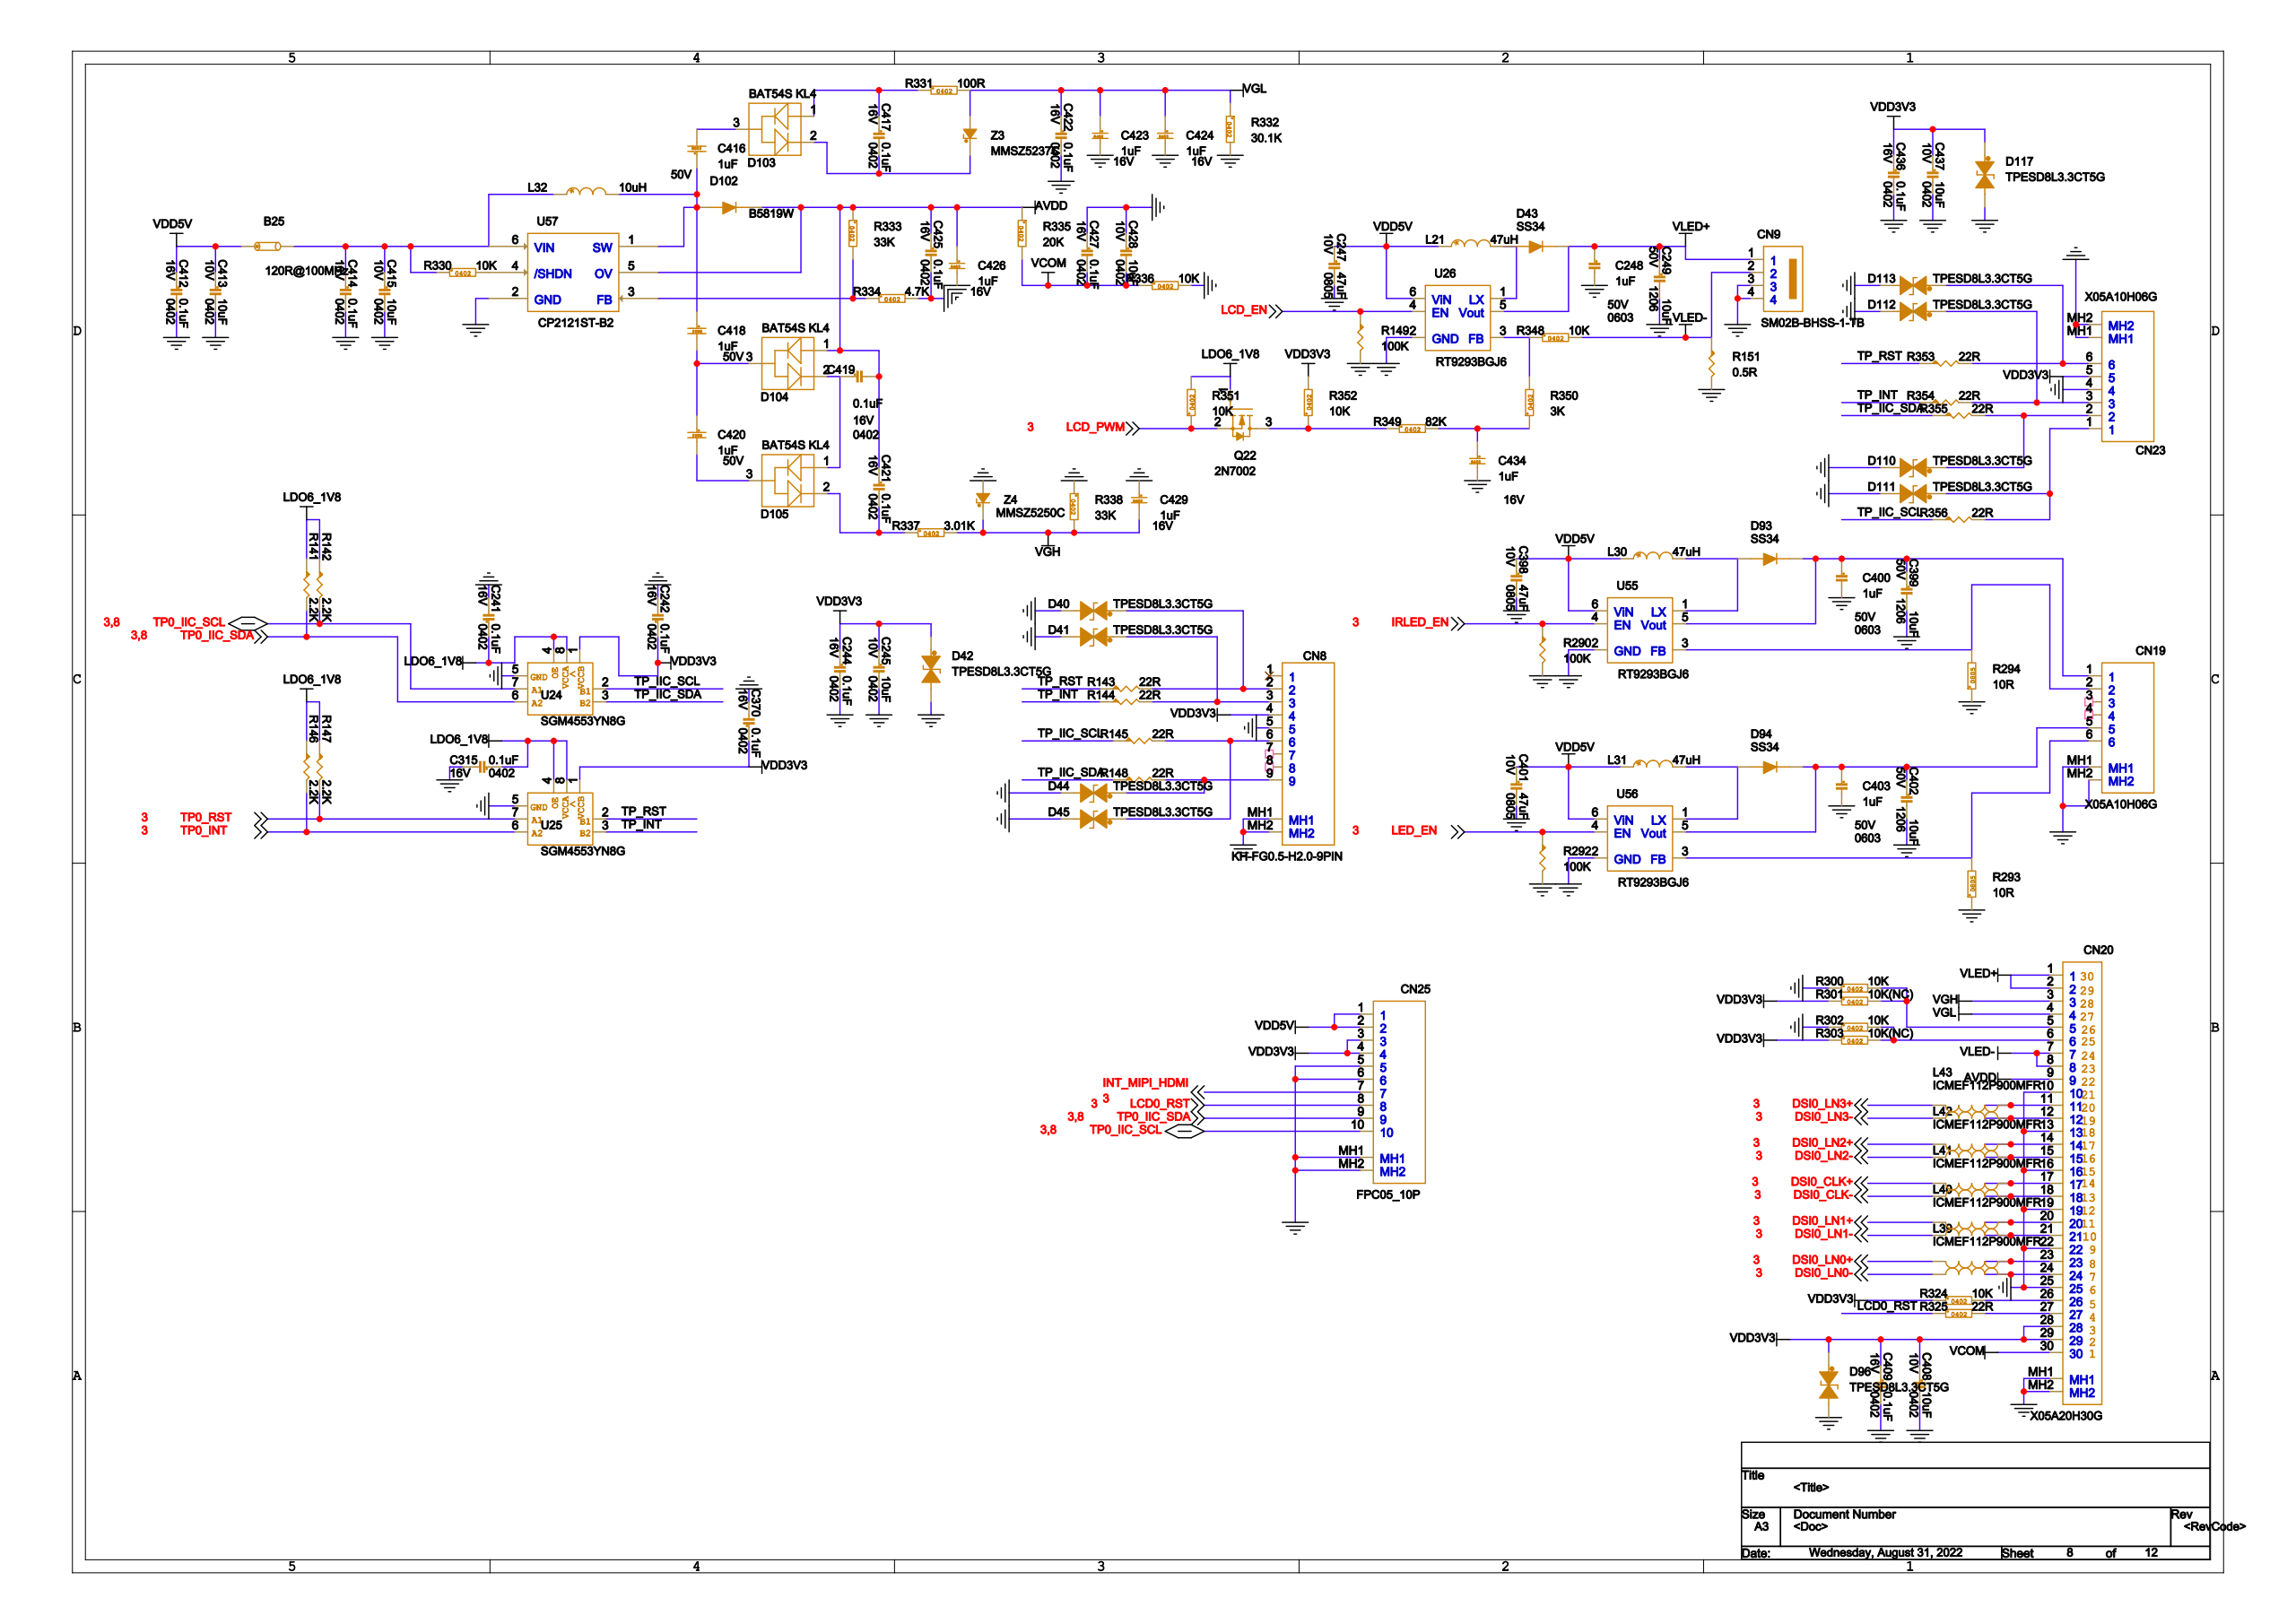Circuit board | Cadence Allegro | 970 parts | 627 nets | one sheet of the schematic
Parts on this sheet (reference | value | footprint):
B25 | 120R@100MHz | R0603
C241 | 0.1uF | C0402
C242 | 0.1uF | C0402
C244 | 0.1uF | C0402
C245 | 10uF | C0402
C247 | 47uF | C0805
C248 | 1uF | C0603
C249 | 10uF | C1206
C315 | 0.1uF | C0402
C370 | 0.1uF | C0402
C398 | 47uF | C0805
C399 | 10uF | C1206
C400 | 1uF | C0603
C401 | 47uF | C0805
C402 | 10uF | C1206
C403 | 1uF | C0603
C408 | 10uF | C0402
C409 | 0.1uF | C0402
C412 | 0.1uF | C0402
C413 | 10uF | C0402
C414 | 0.1uF | C0402
C415 | 10uF | C0402
C416 | 1uF | C0603
C417 | 0.1uF | C0402
C418 | 1uF | C0603
C419 | 0.1uF | C0402
C420 | 1uF | C0603
C421 | 0.1uF | C0402
C422 | 0.1uF | C0402
C423 | 1uF | C0402
C424 | 1uF | C0402
C425 | 0.1uF | C0402
C426 | 1uF | C0402
C427 | 0.1uF | C0402
C428 | 10uF | C0402
C429 | 1uF | C0402
C434 | 1uF | C0402
C436 | 0.1uF | C0402
C437 | 10uF | C0402
CN8 | KH-FG0.5-H2.0-9PIN | FPC-9-0P5-2MMH
CN9 | SM02B-BHSS-1-TB | SM02B
CN19 | X05A10H06G | FPC-6-0P5-2MMH
CN20 | X05A20H30G | FPC-30-0P5-2MMH
CN23 | X05A10H06G | FPC-6-0P5-2MMH
CN25 | FPC05_10P | FPC-10-0P5-2MMH
D40 | TPESD8L3.3CT5G | DFN1006_2L
D41 | TPESD8L3.3CT5G | DFN1006_2L
D42 | TPESD8L3.3CT5G | DFN1006_2L
D43 | SS34 | SMA
D44 | TPESD8L3.3CT5G | DFN1006_2L
D45 | TPESD8L3.3CT5G | DFN1006_2L
D93 | SS34 | SMA
D94 | SS34 | SMA
D96 | TPESD8L3.3CT5G | DFN1006_2L
D102 | B5819W | SOD-123
D103 | BAT54S KL4 | SOT-23
D104 | BAT54S KL4 | SOT-23
D105 | BAT54S KL4 | SOT-23
D110 | TPESD8L3.3CT5G | DFN1006_2L
D111 | TPESD8L3.3CT5G | DFN1006_2L
D112 | TPESD8L3.3CT5G | DFN1006_2L
D113 | TPESD8L3.3CT5G | DFN1006_2L
D117 | TPESD8L3.3CT5G | DFN1006_2L
L21 | 47uH | IND5X5
L30 | 47uH | IND5X5
L31 | 47uH | IND5X5
L32 | 10uH | L4018
L39 | ICMEF112P900MFR | ICMEF112P900MFR
L40 | ICMEF112P900MFR | ICMEF112P900MFR
L41 | ICMEF112P900MFR | ICMEF112P900MFR
L42 | ICMEF112P900MFR | ICMEF112P900MFR
L43 | ICMEF112P900MFR | ICMEF112P900MFR
Q22 | 2N7002 | SOT-23
R141 | 2.2K | R0402
R142 | 2.2K | R0402
R143 | 22R | R0402
R144 | 22R | R0402
R145 | 22R | R0402
R146 | 2.2K | R0402
R147 | 2.2K | R0402
R148 | 22R | R0402
R149 | 100K | R0402
R151 | 0.5R | R1210
R290 | 100K | R0402
R292 | 100K | R0402
R293 | 10R | R0805
R294 | 10R | R0805
R300 | 10K | R0402
R301 | 10K(NC) | R0402
R302 | 10K | R0402
R303 | 10K(NC) | R0402
R324 | 10K | R0402
R325 | 22R | R0402
R330 | 10K | R0402
R331 | 100R | R0402
R332 | 30.1K | R0402
R333 | 33K | R0402
R334 | 4.7K | R0402
R335 | 20K | R0402
R336 | 10K | R0402
R337 | 3.01K | R0402
R338 | 33K | R0402
R348 | 10K | R0402
R349 | 82K | R0402
R350 | 3K | R0402
R351 | 10K | R0402
R352 | 10K | R0402
R353 | 22R | R0402
R354 | 22R | R0402
R355 | 22R | R0402
R356 | 22R | R0402
U24 | SGM4553YN8G | SOT23_8
U25 | SGM4553YN8G | SOT23_8
U26 | RT9293BGJ6 | SOT23-6
U55 | RT9293BGJ6 | SOT23-6
U56 | RT9293BGJ6 | SOT23-6
U57 | CP2121ST-B2 | SOT23-6
Z3 | MMSZ5237C | SOD-123
Z4 | MMSZ5250C | SOD-123
Nets of these parts (net: part-pin ...):
VDD5V: B25-1 C247-1 C398-1 C401-1 C412-1 C413-1 CN25-1 CN25-2 L21-1 L30-1 L31-1 U26-6 U55-6 U56-6
TP0_IIC_SCL: CN25-10 R142-2 U24-7
VDD3V3: C242-1 C244-1 C245-1 C370-1 C408-1 C409-1 C436-1 C437-1 CN8-4 CN23-5 CN25-3 CN25-4 D42-2 D96-2 D117-2 R301-1 R303-1 R324-1 R352-2 U24-1 U25-1 CN20-28 CN20-29
GND: C241-2 C242-2 C244-2 C245-2 C247-2 C248-2 C249-2 C315-2 C370-2 C398-2 C399-2 C400-2 C401-2 C402-2 C403-2 C408-2 C409-2 C412-2 C413-2 C414-2 C415-2 C422-2 C423-2 C424-2 C425-2 C426-2 C427-1 C428-1 C429-1 C434-2 C436-2 C437-2 CN8-5 CN8-MH1 CN8-MH2 CN9-3 CN9-4 CN19-MH1 CN19-MH2 CN23-4 CN23-MH1 CN23-MH2 CN25-5 CN25-6 CN25-MH1 CN25-MH2 D40-1 D41-1 D42-1 D44-1 D45-1 D96-1 D110-1 D111-1 D112-1 D113-1 D117-1 L39-5 L39-6 L40-5 L40-6 L41-5 L41-6 L42-5 L42-6 L43-5 L43-6 R149-2 R151-2 R290-2 R292-2 R293-1 R294-1 R300-1 R302-1 R332-2 R334-2 R336-2 R338-1 U24-5 U25-5 U26-2 U55-2 U56-2 U57-2 Z4-1 CN20-10 CN20-13 CN20-16 CN20-19 CN20-22 CN20-25 CN20-MH1 CN20-MH2
INT_MIPI_HDMI: CN25-7
LCD0_RST: CN25-8 R325-1
TP0_IIC_SDA: CN25-9 R141-2 U24-6
N19701757: R300-2 R301-2 CN20-5
N19701754: R302-2 R303-2 CN20-6
N19775943: CN23-1 D111-2 R356-2
N19775935: CN23-2 D110-2 R355-2
N19775912: CN23-3 D112-2 R354-2
N19775902: CN23-6 D113-2 R353-2
N19693294: C399-1 C400-1 CN19-1 D93-2 U55-5
N19693252: CN19-2 R294-2 U55-3
N19693946: C402-1 C403-1 CN19-5 D94-2 U56-5
N19693904: CN19-6 R293-2 U56-3
N19773504: Q22-3 R349-1 R352-1
LDO6_1V8: C241-1 C315-1 Q22-1 R141-1 R142-1 R146-1 R147-1 R351-2 U24-4 U24-8 U25-4 U25-8
LCD_PWM: Q22-2 R351-1
N19773224: C434-1 R349-2 R350-1
N19411041: R348-1 R350-2 U26-3
N19716318: B25-2 C414-1 C415-1 L32-1 R330-1 U57-6
N19717157: C416-1 C418-1 D102-1 L32-2 U57-1
N19728237: C416-2 D103-3
N19728347: C418-2 C420-1 D104-3
N19728874: C420-2 D105-3
VLED+: C248-1 C249-1 CN9-1 D43-2 U26-5 CN20-1 CN20-2
N19703327: L43-1 CN20-11
N19703330: L43-2 CN20-12
N19703455: L42-1 CN20-14
N19703458: L42-2 CN20-15
N19703600: L41-1 CN20-17
N19703603: L41-2 CN20-18
N19703747: L40-1 CN20-20
N19703750: L40-2 CN20-21
N19703897: L39-1 CN20-23
N19703900: L39-2 CN20-24
N19704133: R324-2 CN20-26
N19704199: R325-2 CN20-27
VGH: C429-2 R337-2 R338-2 Z4-2 CN20-3
VCOM: C427-2 C428-2 R335-2 R336-1 CN20-30
VGL: C422-1 C423-1 C424-1 R331-2 R332-1 Z3-1 CN20-4
VLED-: CN9-2 R151-1 R348-2 CN20-7 CN20-8
AVDD: C419-2 C421-1 C425-1 C426-1 D102-2 D104-2 R333-1 R335-1 U57-5 CN20-9
N19728266: C417-2 D103-1 Z3-2
N19728257: C417-1 D103-2 R331-1
N19728889: C419-1 D104-1 D105-2
N19728891: C421-2 D105-1 R337-1
N197165973: R330-2 U57-4
N19730194: R333-2 R334-1 U57-3
N19693286: D93-1 L30-2 U55-1
N19693938: D94-1 L31-2 U56-1
N19410922: D43-1 L21-2 U26-1
DSI0_LN0+: L39-3
DSI0_LN0-: L39-4
DSI0_LN1+: L40-3
DSI0_LN1-: L40-4
DSI0_CLK+: L41-3
DSI0_CLK-: L41-4
DSI0_LN2+: L42-3
DSI0_LN2-: L42-4
DSI0_LN3+: L43-3
DSI0_LN3-: L43-4
IRLED_EN: R290-1 U55-4
LED_EN: R292-1 U56-4
LCD_EN: R149-1 U26-4
N19303977: CN8-2 D40-2 R143-2
N19303998: CN8-3 D41-2 R144-2
N19304267: CN8-6 D45-2 R145-2
N19304230: CN8-9 D44-2 R148-2
TP_RST: R143-1 R353-1 U25-2
TP_INT: R144-1 R354-1 U25-3
TP_IIC_SDA: R148-1 R355-1 U24-3
TP_IIC_SCL: R145-1 R356-1 U24-2
TP0_INT: R146-2 U25-6
TP0_RST: R147-2 U25-7